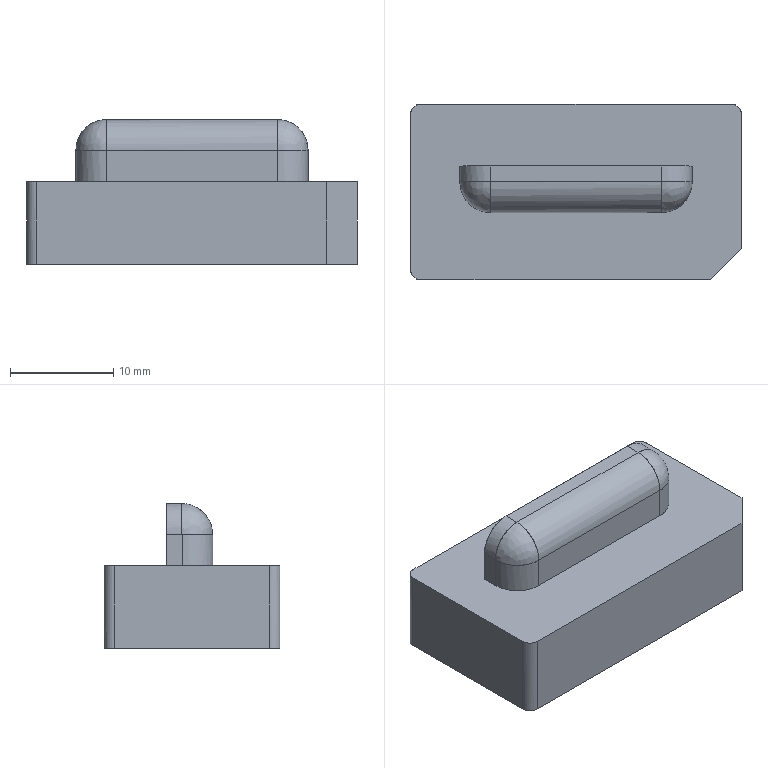NC program | PowerMill | posted with a generic post | part box 32 x 17 x 14 mm
Lines 6119 to 6787 of 64476:
N6216 M6
N6217 S8500 M03
N6218 G00 G90 X0.0 Y0.0
N6219 G43 Z9.8 H3
N6220
N6221 G05 P10000 R8
N6222 X21.8229 Y17.0704
N6223 Z-5.0
N6224 G01 Z-6.2 F360.0
N6225 X18.8213 Y12.7327 F600.0
N6226 X9.1162 Y7.8802
N6227 X11.2546
N6228 X11.536 Y7.8712
N6229 X11.8173 Y7.8475
N6230 X12.0987 Y7.8089
N6231 X12.3801 Y7.7548
N6232 X12.7815 Y7.6502
N6233 X12.9428 Y7.5988
N6234 X13.2242 Y7.4952
N6235 X13.5055 Y7.3733
N6236 X13.7743 Y7.2382
N6237 X14.0683 Y7.0681
N6238 X14.3496 Y6.8803
N6239 X14.631 Y6.6655
N6240 X14.8049 Y6.5169
N6241 X14.9993 Y6.3348
N6242 X15.1937 Y6.1334
N6243 X15.3539 Y5.9502
N6244 X15.5687 Y5.6758
N6245 X15.768 Y5.3835
N6246 X15.936 Y5.1002
N6247 X16.0815 Y4.8168
N6248 X16.2069 Y4.5335
N6249 X16.3134 Y4.2501
N6250 X16.4047 Y3.9581
N6251 X16.4742 Y3.6834
N6252 X16.5302 Y3.4001
N6253 X16.5703 Y3.1168
N6254 X16.5955 Y2.8334
N6255 X16.6058 Y2.5501
N6256 X16.6052 Y0.85
N6257 X16.5972 Y0.5667
N6258 X16.5791 Y0.2833
N6259 X16.514 Y-0.2833
N6260 X16.4666 Y-0.5667
N6261 X16.409 Y-0.85
N6262 X16.3192 Y-1.2164
N6263 X16.2626 Y-1.4167
N6264 X16.1729 Y-1.7001
N6265 X16.0724 Y-1.9834
N6266 X15.9599 Y-2.2667
N6267 X15.8348 Y-2.5501
N6268 X15.7565 Y-2.7144
N6269 X15.5457 Y-3.1168
N6270 X15.3798 Y-3.4001
N6271 X15.1937 Y-3.6904
N6272 X14.9976 Y-3.9702
N6273 X14.7832 Y-4.2501
N6274 X14.6265 Y-4.4405
N6275 X14.4641 Y-4.626
N6276 X14.287 Y-4.8168
N6277 X14.0683 Y-5.0365
N6278 X13.88 Y-5.2129
N6279 X13.6866 Y-5.3835
N6280 X13.5055 Y-5.5337
N6281 X13.2242 Y-5.7509
N6282 X12.9423 Y-5.9502
N6283 X12.6612 Y-6.1323
N6284 X12.3801 Y-6.2988
N6285 X11.9685 Y-6.5169
N6286 X11.8173 Y-6.5896
N6287 X11.536 Y-6.7156
N6288 X11.2546 Y-6.8293
N6289 X10.9732 Y-6.9307
N6290 X10.6919 Y-7.0218
N6291 X10.4781 Y-7.0836
N6292 X10.1291 Y-7.171
N6293 X9.8478 Y-7.2304
N6294 X9.5664 Y-7.2795
N6295 X9.0037 Y-7.3484
N6296 X8.7223 Y-7.3683
N6297 X8.441 Y-7.378
N6298 X-8.441 Y-7.3777
N6299 X-8.7223 Y-7.368
N6300 X-9.0037 Y-7.3481
N6301 X-9.5664 Y-7.2795
N6302 X-10.1291 Y-7.1713
N6303 X-10.4784 Y-7.0836
N6304 X-10.6919 Y-7.0221
N6305 X-10.9732 Y-6.9312
N6306 X-11.2546 Y-6.8293
N6307 X-11.536 Y-6.7156
N6308 X-11.8173 Y-6.5896
N6309 X-11.9682 Y-6.5169
N6310 X-12.3801 Y-6.2988
N6311 X-12.6612 Y-6.1323
N6312 X-12.9428 Y-5.9499
N6313 X-13.2242 Y-5.7509
N6314 X-13.5055 Y-5.5337
N6315 X-13.6938 Y-5.3773
N6316 X-13.8774 Y-5.2155
N6317 X-14.0683 Y-5.0365
N6318 X-14.287 Y-4.8168
N6319 X-14.4643 Y-4.626
N6320 X-14.6266 Y-4.4404
N6321 X-14.7835 Y-4.2501
N6322 X-14.9976 Y-3.9702
N6323 X-15.1984 Y-3.6834
N6324 X-15.3802 Y-3.4001
N6325 X-15.5457 Y-3.1168
N6326 X-15.7565 Y-2.7147
N6327 X-15.8348 Y-2.5501
N6328 X-15.9597 Y-2.2667
N6329 X-16.0724 Y-1.9834
N6330 X-16.1729 Y-1.7001
N6331 X-16.2626 Y-1.4167
N6332 X-16.3192 Y-1.2164
N6333 X-16.409 Y-0.85
N6334 X-16.4667 Y-0.5667
N6335 X-16.514 Y-0.2833
N6336 X-16.5791 Y0.2833
N6337 X-16.5972 Y0.5667
N6338 X-16.6052 Y0.85
N6339 X-16.6058 Y2.5501
N6340 X-16.5957 Y2.8334
N6341 X-16.5703 Y3.1168
N6342 X-16.53 Y3.4001
N6343 X-16.4742 Y3.6834
N6344 X-16.4046 Y3.9581
N6345 X-16.3134 Y4.2501
N6346 X-16.2067 Y4.5335
N6347 X-16.0815 Y4.8168
N6348 X-15.9357 Y5.1002
N6349 X-15.7565 Y5.4015
N6350 X-15.5686 Y5.6758
N6351 X-15.3539 Y5.9502
N6352 X-15.1937 Y6.1334
N6353 X-14.9993 Y6.3348
N6354 X-14.8049 Y6.5169
N6355 X-14.631 Y6.6655
N6356 X-14.3496 Y6.8803
N6357 X-14.043 Y7.0836
N6358 X-13.7743 Y7.2382
N6359 X-13.5055 Y7.3733
N6360 X-13.2242 Y7.4952
N6361 X-12.9428 Y7.5988
N6362 X-12.7815 Y7.6502
N6363 X-12.3801 Y7.7548
N6364 X-12.0987 Y7.8089
N6365 X-11.8173 Y7.8475
N6366 X-11.536 Y7.8712
N6367 X-11.2546 Y7.8802
N6368 X9.1162
N6369 G00 Z9.8
N6370 G05 P0
N6371 (---------------)
N6372 ( END TOOLPATH : 精公基准台01-基准面偏置-D10 )
N6373 (---------------)
N6374 ( START TOOLPATH : 精公基准台01-基准台侧光-D10 )
N6375 (---------------)
N6376 G00 X0.0 Y0.0 Z9.8
N6377 G05 P10000 R8
N6378 X20.98 Y-14.7753
N6379 Z-12.9
N6380 G01 Z-14.1 F360.0
N6381 G03 X17.4444 Y-11.2398 I-1.7678 J1.7677 F600.0
N6382 G01 X16.6141 Y-12.0701
N6383 X16.6138 Y-12.0704
N6384 X16.6135 Y-12.0707
N6385 X16.4955 Y-12.1861
N6386 X16.4942 Y-12.1874
N6387 X16.4928 Y-12.1887
N6388 X16.2678 Y-12.3894
N6389 X16.2666 Y-12.3905
N6390 X16.2653 Y-12.3916
N6391 X16.1741 Y-12.4663
N6392 X16.1725 Y-12.4675
N6393 X16.1709 Y-12.4688
N6394 X15.8548 Y-12.7019
N6395 X15.8523 Y-12.7037
N6396 X15.8497 Y-12.7054
N6397 X15.5336 Y-12.9031
N6398 X15.531 Y-12.9046
N6399 X15.5285 Y-12.906
N6400 X15.2123 Y-13.0729
N6401 X15.2098 Y-13.0742
N6402 X15.2073 Y-13.0754
N6403 X14.8911 Y-13.2148
N6404 X14.8884 Y-13.216
N6405 X14.8855 Y-13.2171
N6406 X14.4996 Y-13.3535
N6407 X14.4971 Y-13.3544
N6408 X14.4946 Y-13.3551
N6409 X14.2482 Y-13.4243
N6410 X14.2459 Y-13.4249
N6411 X14.2437 Y-13.4254
N6412 X13.9275 Y-13.4946
N6413 X13.925 Y-13.4951
N6414 X13.9225 Y-13.4955
N6415 X13.6063 Y-13.5437
N6416 X13.6038 Y-13.544
N6417 X13.6012 Y-13.5443
N6418 X13.2851 Y-13.572
N6419 X13.2826 Y-13.5721
N6420 X13.2801 Y-13.5722
N6421 X12.9639 Y-13.58
N6422 X12.963
N6423 X12.962
N6424 X-14.8588
N6425 X-14.8592
N6426 X-14.8596
N6427 X-15.1758 Y-13.577
N6428 X-15.1775 Y-13.5769
N6429 X-15.1793 Y-13.5768
N6430 X-15.4955 Y-13.5597
N6431 X-15.4976 Y-13.5596
N6432 X-15.4998 Y-13.5594
N6433 X-15.8159 Y-13.525
N6434 X-15.8181 Y-13.5247
N6435 X-15.8202 Y-13.5244
N6436 X-16.1363 Y-13.4728
N6437 X-16.1384 Y-13.4724
N6438 X-16.1405 Y-13.472
N6439 X-16.4567 Y-13.4029
N6440 X-16.4588 Y-13.4024
N6441 X-16.4609 Y-13.4018
N6442 X-16.777 Y-13.3145
N6443 X-16.7792 Y-13.3139
N6444 X-16.7814 Y-13.3132
N6445 X-17.0975 Y-13.2061
N6446 X-17.0995 Y-13.2054
N6447 X-17.1015 Y-13.2046
N6448 X-17.4176 Y-13.0786
N6449 X-17.4199 Y-13.0776
N6450 X-17.4221 Y-13.0766
N6451 X-17.7382 Y-12.9277
N6452 X-17.7402 Y-12.9267
N6453 X-17.7422 Y-12.9257
N6454 X-18.0584 Y-12.7548
N6455 X-18.0605 Y-12.7535
N6456 X-18.0627 Y-12.7522
N6457 X-18.3788 Y-12.5546
N6458 X-18.3807 Y-12.5535
N6459 X-18.3824 Y-12.5523
N6460 X-18.606 Y-12.3951
N6461 X-18.6071 Y-12.3944
N6462 X-18.6081 Y-12.3936
N6463 X-18.7007 Y-12.3241
N6464 X-18.702 Y-12.323
N6465 X-18.7033 Y-12.322
N6466 X-19.004 Y-12.0754
N6467 X-19.0061 Y-12.0736
N6468 X-19.0082 Y-12.0717
N6469 X-19.3399 Y-11.758
N6470 X-19.342 Y-11.7559
N6471 X-19.344 Y-11.7537
N6472 X-19.6341 Y-11.4351
N6473 X-19.6358 Y-11.4331
N6474 X-19.6376 Y-11.431
N6475 X-19.8886 Y-11.1148
N6476 X-19.8898 Y-11.1133
N6477 X-19.891 Y-11.1117
N6478 X-19.9822 Y-10.9845
N6479 X-19.9829 Y-10.9835
N6480 X-19.9836 Y-10.9824
N6481 X-20.1103 Y-10.7935
N6482 X-20.1114 Y-10.7919
N6483 X-20.1124 Y-10.7902
N6484 X-20.3018 Y-10.4758
N6485 X-20.3031 Y-10.4737
N6486 X-20.3042 Y-10.4715
N6487 X-20.4703 Y-10.1537
N6488 X-20.4713 Y-10.1516
N6489 X-20.4723 Y-10.1495
N6490 X-20.6144 Y-9.8333
N6491 X-20.6153 Y-9.8312
N6492 X-20.6162 Y-9.8291
N6493 X-20.737 Y-9.5129
N6494 X-20.7378 Y-9.5108
N6495 X-20.7385 Y-9.5087
N6496 X-20.8396 Y-9.1926
N6497 X-20.8403 Y-9.1905
N6498 X-20.8408 Y-9.1884
N6499 X-20.9231 Y-8.8722
N6500 X-20.9236 Y-8.87
N6501 X-20.9241 Y-8.8678
N6502 X-20.9876 Y-8.5517
N6503 X-20.988 Y-8.5498
N6504 X-20.9883 Y-8.5478
N6505 X-21.0357 Y-8.2317
N6506 X-21.036 Y-8.2294
N6507 X-21.0363 Y-8.2271
N6508 X-21.0653 Y-7.911
N6509 X-21.0655 Y-7.909
N6510 X-21.0656 Y-7.9071
N6511 X-21.0792 Y-7.5909
N6512 Y-7.5892
N6513 Y-7.5875
N6514 Y7.5875
N6515 Y7.5891
N6516 Y7.5907
N6517 X-21.0664 Y7.9069
N6518 X-21.0662 Y7.909
N6519 X-21.0661 Y7.9112
N6520 X-21.0363 Y8.2273
N6521 X-21.036 Y8.2294
N6522 X-21.0358 Y8.2315
N6523 X-20.989 Y8.5476
N6524 X-20.9887 Y8.5494
N6525 X-20.9884 Y8.5513
N6526 X-20.9441 Y8.7781
N6527 X-20.9437 Y8.7802
N6528 X-20.9432 Y8.7823
N6529 X-20.8409 Y9.1878
N6530 X-20.8402 Y9.1902
N6531 X-20.8395 Y9.1926
N6532 X-20.7384 Y9.5087
N6533 X-20.7377 Y9.5108
N6534 X-20.737 Y9.5128
N6535 X-20.6243 Y9.8095
N6536 X-20.6234 Y9.8117
N6537 X-20.6225 Y9.8138
N6538 X-20.4722 Y10.1494
N6539 X-20.4712 Y10.1515
N6540 X-20.4701 Y10.1537
N6541 X-20.3052 Y10.4698
N6542 X-20.304 Y10.4719
N6543 X-20.3028 Y10.4741
N6544 X-20.1126 Y10.7902
N6545 X-20.1116 Y10.7919
N6546 X-20.1105 Y10.7935
N6547 X-19.9836 Y10.9828
N6548 X-19.9829 Y10.9839
N6549 X-19.9821 Y10.9849
N6550 X-19.8909 Y11.1118
N6551 X-19.8899 Y11.1132
N6552 X-19.8888 Y11.1146
N6553 X-19.6639 Y11.4005
N6554 X-19.6622 Y11.4027
N6555 X-19.6603 Y11.4048
N6556 X-19.3466 Y11.7511
N6557 X-19.3445 Y11.7533
N6558 X-19.3424 Y11.7554
N6559 X-19.0238 Y12.0578
N6560 X-19.0217 Y12.0598
N6561 X-19.0196 Y12.0616
N6562 X-18.7034 Y12.3219
N6563 X-18.7021 Y12.323
N6564 X-18.7007 Y12.3241
N6565 X-18.6081 Y12.3936
N6566 X-18.607 Y12.3945
N6567 X-18.6058 Y12.3953
N6568 X-18.3822 Y12.5513
N6569 X-18.3809 Y12.5523
N6570 X-18.3795 Y12.5532
N6571 X-18.1285 Y12.7133
N6572 X-18.1263 Y12.7146
N6573 X-18.1241 Y12.7159
N6574 X-17.7428 Y12.9261
N6575 X-17.7405 Y12.9273
N6576 X-17.7381 Y12.9285
N6577 X-17.422 Y13.0767
N6578 X-17.4199 Y13.0776
N6579 X-17.4178 Y13.0785
N6580 X-17.1016 Y13.2052
N6581 X-17.0995 Y13.206
N6582 X-17.0974 Y13.2068
N6583 X-16.7812 Y13.3131
N6584 X-16.7791 Y13.3138
N6585 X-16.777 Y13.3144
N6586 X-16.4609 Y13.4018
N6587 X-16.4588 Y13.4023
N6588 X-16.4566 Y13.4028
N6589 X-16.1405 Y13.4718
N6590 X-16.1384 Y13.4722
N6591 X-16.1364 Y13.4726
N6592 X-15.8202 Y13.5244
N6593 X-15.8181 Y13.5247
N6594 X-15.8159 Y13.525
N6595 X-15.4997 Y13.5591
N6596 X-15.4976 Y13.5593
N6597 X-15.4955 Y13.5595
N6598 X-15.1794 Y13.5768
N6599 X-15.1776 Y13.5769
N6600 X-15.1758
N6601 X-14.8596 Y13.58
N6602 X-14.8592
N6603 X-14.8588
N6604 X0.0
N6605 X14.8588
N6606 X14.8592
N6607 X14.8596
N6608 X15.1758 Y13.577
N6609 X15.1775 Y13.5769
N6610 X15.1793 Y13.5768
N6611 X15.4955 Y13.5597
N6612 X15.4976 Y13.5596
N6613 X15.4998 Y13.5594
N6614 X15.8159 Y13.525
N6615 X15.8181 Y13.5247
N6616 X15.8202 Y13.5244
N6617 X16.1363 Y13.4728
N6618 X16.1384 Y13.4724
N6619 X16.1405 Y13.472
N6620 X16.4567 Y13.4029
N6621 X16.4588 Y13.4024
N6622 X16.4609 Y13.4018
N6623 X16.777 Y13.3145
N6624 X16.7792 Y13.3139
N6625 X16.7814 Y13.3132
N6626 X17.0975 Y13.2061
N6627 X17.0995 Y13.2054
N6628 X17.1015 Y13.2046
N6629 X17.4176 Y13.0786
N6630 X17.4199 Y13.0776
N6631 X17.4221 Y13.0766
N6632 X17.7382 Y12.9277
N6633 X17.7402 Y12.9267
N6634 X17.7422 Y12.9257
N6635 X18.0584 Y12.7548
N6636 X18.0605 Y12.7535
N6637 X18.0627 Y12.7522
N6638 X18.3788 Y12.5546
N6639 X18.3807 Y12.5535
N6640 X18.3824 Y12.5523
N6641 X18.606 Y12.3951
N6642 X18.6071 Y12.3944
N6643 X18.6081 Y12.3936
N6644 X18.7007 Y12.3241
N6645 X18.702 Y12.323
N6646 X18.7033 Y12.322
N6647 X19.004 Y12.0754
N6648 X19.0061 Y12.0736
N6649 X19.0082 Y12.0717
N6650 X19.3399 Y11.758
N6651 X19.342 Y11.7559
N6652 X19.344 Y11.7537
N6653 X19.6341 Y11.4351
N6654 X19.6358 Y11.4331
N6655 X19.6376 Y11.431
N6656 X19.8886 Y11.1148
N6657 X19.8898 Y11.1133
N6658 X19.891 Y11.1117
N6659 X19.9822 Y10.9845
N6660 X19.9829 Y10.9835
N6661 X19.9836 Y10.9824
N6662 X20.1103 Y10.7935
N6663 X20.1114 Y10.7919
N6664 X20.1124 Y10.7902
N6665 X20.3018 Y10.4758
N6666 X20.3031 Y10.4737
N6667 X20.3042 Y10.4715
N6668 X20.4703 Y10.1537
N6669 X20.4713 Y10.1516
N6670 X20.4723 Y10.1495
N6671 X20.6144 Y9.8333
N6672 X20.6153 Y9.8312
N6673 X20.6162 Y9.8291
N6674 X20.737 Y9.5129
N6675 X20.7378 Y9.5108
N6676 X20.7385 Y9.5087
N6677 X20.8396 Y9.1926
N6678 X20.8403 Y9.1905
N6679 X20.8408 Y9.1884
N6680 X20.9231 Y8.8722
N6681 X20.9236 Y8.87
N6682 X20.9241 Y8.8678
N6683 X20.9876 Y8.5517
N6684 X20.988 Y8.5498
N6685 X20.9883 Y8.5478
N6686 X21.0357 Y8.2317
N6687 X21.036 Y8.2294
N6688 X21.0363 Y8.2271
N6689 X21.0653 Y7.911
N6690 X21.0655 Y7.909
N6691 X21.0656 Y7.9071
N6692 X21.0792 Y7.5909
N6693 Y7.5892
N6694 Y7.5875
N6695 X21.08 Y-5.3745
N6696 Y-5.3749
N6697 Y-5.3754
N6698 X21.0764 Y-5.6915
N6699 X21.0763 Y-5.6939
N6700 X21.0762 Y-5.6962
N6701 X21.0541 Y-6.0124
N6702 X21.0538 Y-6.0149
N6703 X21.0535 Y-6.0174
N6704 X21.0111 Y-6.3336
N6705 X21.0107 Y-6.3361
N6706 X21.0103 Y-6.3386
N6707 X20.947 Y-6.6548
N6708 X20.9464 Y-6.6573
N6709 X20.9458 Y-6.6598
N6710 X20.8608 Y-6.976
N6711 X20.8601 Y-6.9785
N6712 X20.8593 Y-6.981
N6713 X20.7514 Y-7.2972
N6714 X20.7505 Y-7.2997
N6715 X20.7496 Y-7.3021
N6716 X20.6233 Y-7.605
N6717 X20.6222 Y-7.6075
N6718 X20.621 Y-7.6101
N6719 X20.4559 Y-7.9395
N6720 X20.4545 Y-7.9421
N6721 X20.453 Y-7.9447
N6722 X20.2643 Y-8.2608
N6723 X20.2627 Y-8.2634
N6724 X20.261 Y-8.2659
N6725 X20.0382 Y-8.582
N6726 X20.0371 Y-8.5836
N6727 X20.0359 Y-8.5851
N6728 X19.9803 Y-8.6565
N6729 X19.9793 Y-8.6578
N6730 X19.9782 Y-8.6591
N6731 X19.771 Y-8.9038
N6732 X19.7697 Y-8.9052
N6733 X19.7684 Y-8.9067
N6734 X19.6595 Y-9.0234
N6735 X19.6587 Y-9.0243
N6736 X19.6578 Y-9.0252
N6737 X19.4596 Y-9.2246
N6738 X19.4595 Y-9.2247
N6739 X19.4594 Y-9.2248
N6740 X17.4444 Y-11.2398
N6741 G03 X20.98 Y-14.7753 I1.7678 J-1.7678
N6742 G01 X20.9285 Y-14.7137
N6743 G03 X17.393 Y-11.1781 I-1.7678 J1.7678
N6744 G01 X16.5575 Y-12.0135
N6745 X16.4396 Y-12.129
N6746 X16.2146 Y-12.3297
N6747 X16.1234 Y-12.4044
N6748 X15.8073 Y-12.6375
N6749 X15.4911 Y-12.8352
N6750 X15.175 Y-13.0022
N6751 X14.8588 Y-13.1416
N6752 X14.473 Y-13.2781
N6753 X14.2266 Y-13.3472
N6754 X13.9104 Y-13.4164
N6755 X13.5943 Y-13.4646
N6756 X13.2781 Y-13.4923
N6757 X12.962 Y-13.5
N6758 X-14.8588
N6759 X-15.175 Y-13.497
N6760 X-15.4911 Y-13.4799
N6761 X-15.8073 Y-13.4454
N6762 X-16.1234 Y-13.3938
N6763 X-16.4396 Y-13.3247
N6764 X-16.7557 Y-13.2374
N6765 X-17.0719 Y-13.1303
N6766 X-17.388 Y-13.0043
N6767 X-17.7042 Y-12.8553
N6768 X-18.0203 Y-12.6844
N6769 X-18.3364 Y-12.4868
N6770 X-18.56 Y-12.3297
N6771 X-18.6526 Y-12.2601
N6772 X-18.9532 Y-12.0135
N6773 X-19.2849 Y-11.6999
N6774 X-19.5749 Y-11.3812
N6775 X-19.8259 Y-11.0651
N6776 X-19.9172 Y-10.9379
N6777 X-20.0439 Y-10.749
N6778 X-20.2333 Y-10.4345
N6779 X-20.3993 Y-10.1167
N6780 X-20.5415 Y-9.8005
N6781 X-20.6623 Y-9.4844
N6782 X-20.7634 Y-9.1682
N6783 X-20.8457 Y-8.8521
N6784 X-20.9092 Y-8.5359
N6785 X-20.9566 Y-8.2198
N6786 X-20.9857 Y-7.9036
N6787 X-20.9992 Y-7.5875
N6788 X-21.0 Y-7.2714
N6789 Y7.2714
N6790 X-20.9992 Y7.5875
N6791 X-20.9864 Y7.9036
N6792 X-20.9566 Y8.2198
N6793 X-20.9099 Y8.5359
N6794 X-20.8656 Y8.7628
N6795 X-20.7633 Y9.1682
N6796 X-20.6622 Y9.4844
N6797 X-20.5495 Y9.7811
N6798 X-20.3992 Y10.1167
N6799 X-20.2343 Y10.4328
N6800 X-20.044 Y10.749
N6801 X-19.9172 Y10.9382
N6802 X-19.8259 Y11.0651
N6803 X-19.601 Y11.3511
N6804 X-19.2873 Y11.6974
N6805 X-18.9687 Y11.9998
N6806 X-18.6526 Y12.2601
N6807 X-18.56 Y12.3297
N6808 X-18.3364 Y12.4857
N6809 X-18.0854 Y12.6458
N6810 X-17.7042 Y12.856
N6811 X-17.388 Y13.0043
N6812 X-17.0719 Y13.1309
N6813 X-16.7557 Y13.2373
N6814 X-16.4396 Y13.3246
N6815 X-16.1234 Y13.3936
N6816 X-15.8073 Y13.4454
N6817 X-15.4911 Y13.4796
N6818 X-15.175 Y13.4969
N6819 X-14.8588 Y13.5
N6820 X0.0
N6821 X14.8588
N6822 X15.175 Y13.497
N6823 X15.4911 Y13.4799
N6824 X15.8073 Y13.4454
N6825 X16.1234 Y13.3939
N6826 X16.4396 Y13.3247
N6827 X16.7557 Y13.2374
N6828 X17.0719 Y13.1303
N6829 X17.388 Y13.0043
N6830 X17.7042 Y12.8553
N6831 X18.0203 Y12.6844
N6832 X18.3364 Y12.4868
N6833 X18.56 Y12.3297
N6834 X18.6526 Y12.2601
N6835 X18.9532 Y12.0135
N6836 X19.2849 Y11.6999
N6837 X19.5749 Y11.3812
N6838 X19.8259 Y11.0651
N6839 X19.9172 Y10.9379
N6840 X20.0439 Y10.749
N6841 X20.2333 Y10.4345
N6842 X20.3993 Y10.1167
N6843 X20.5415 Y9.8005
N6844 X20.6623 Y9.4844
N6845 X20.7634 Y9.1682
N6846 X20.8457 Y8.8521
N6847 X20.9092 Y8.5359
N6848 X20.9566 Y8.2198
N6849 X20.9857 Y7.9036
N6850 X20.9992 Y7.5875
N6851 X21.0 Y7.2714
N6852 Y-5.3745
N6853 X20.9964 Y-5.6906
N6854 X20.9743 Y-6.0068
N6855 X20.9318 Y-6.3229
N6856 X20.8685 Y-6.6391
N6857 X20.7836 Y-6.9552
N6858 X20.6757 Y-7.2714
N6859 X20.5495 Y-7.5742
N6860 X20.3844 Y-7.9036
N6861 X20.1956 Y-8.2198
N6862 X19.9728 Y-8.5359
N6863 X19.9172 Y-8.6074
N6864 X19.7099 Y-8.8521
N6865 X19.601 Y-8.9688
N6866 X19.4029 Y-9.1682
N6867 X17.393 Y-11.1781
N6868 G03 X20.9285 Y-14.7137 I1.7677 J-1.7678
N6869 G00 Z9.8
N6870 G05 P0
N6871 (---------------)
N6872 ( END TOOLPATH : 精公基准台01-基准台侧光-D10 )
N6873 (---------------)
N6874
N6875 M05
N6876 G53 Z0.0
N6877 (---------------)
N6878 ( START TOOLPATH : 精公精光01-平行-R1.5 )
N6879 (---------------)
N6880 ( TOOL NO.    :22 )
N6881 ( TOOL TYPE   : BALLNOSED)
N6882 ( TOOL ID     : R1.5_1_1)
N6883 ( TOOL DIA    : 3.0 LENGTH 59.88)
N6884 T22